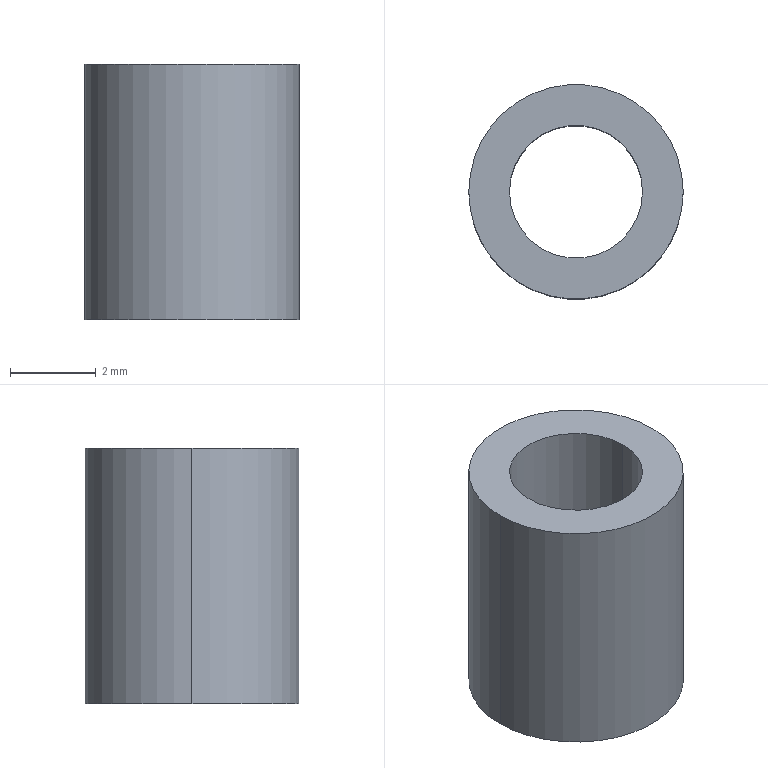Part | SolidWorks | features Extrusion 1 | 1 solid | 6 faces | box 5 x 5 x 5.95 mm | volume 71.919 mm3 | cylinder 4 | plane 2 | commonest cylinder face diameters 3.1 x2 5 x2
STEP:
#1=CARTESIAN_POINT('',(-1.55,0.,5.95));
#2=VERTEX_POINT('',#1);
#3=CARTESIAN_POINT('',(1.55,0.,5.95));
#4=VERTEX_POINT('',#3);
#5=CARTESIAN_POINT('',(0.,0.,5.95));
#6=DIRECTION('',(0.,0.,1.));
#7=DIRECTION('',(1.,0.,0.));
#8=AXIS2_PLACEMENT_3D('',#5,#6,#7);
#9=CIRCLE('',#8,1.55);
#10=EDGE_CURVE('',#2,#4,#9,.T.);
#11=ORIENTED_EDGE('',*,*,#10,.T.);
#12=CARTESIAN_POINT('',(1.55,0.,0.));
#13=VERTEX_POINT('',#12);
#14=CARTESIAN_POINT('',(1.55,0.,5.95));
#15=DIRECTION('',(0.,0.,-1.));
#16=VECTOR('',#15,1000.);
#17=LINE('',#14,#16);
#18=EDGE_CURVE('',#4,#13,#17,.T.);
#19=ORIENTED_EDGE('',*,*,#18,.T.);
#20=CARTESIAN_POINT('',(-1.55,0.,0.));
#21=VERTEX_POINT('',#20);
#22=CARTESIAN_POINT('',(0.,0.,0.));
#23=DIRECTION('',(0.,0.,1.));
#24=DIRECTION('',(1.,0.,0.));
#25=AXIS2_PLACEMENT_3D('',#22,#23,#24);
#26=CIRCLE('',#25,1.55);
#27=EDGE_CURVE('',#21,#13,#26,.T.);
#28=ORIENTED_EDGE('',*,*,#27,.F.);
#29=CARTESIAN_POINT('',(-1.55,0.,5.95));
#30=DIRECTION('',(0.,0.,-1.));
#31=VECTOR('',#30,1000.);
#32=LINE('',#29,#31);
#33=EDGE_CURVE('',#2,#21,#32,.T.);
#34=ORIENTED_EDGE('',*,*,#33,.F.);
#35=EDGE_LOOP('',(#11,#19,#28,#34));
#36=FACE_OUTER_BOUND('',#35,.T.);
#37=CARTESIAN_POINT('',(0.,0.,5.95));
#38=DIRECTION('',(0.,0.,-1.));
#39=DIRECTION('',(-1.,0.,0.));
#40=AXIS2_PLACEMENT_3D('',#37,#38,#39);
#41=CYLINDRICAL_SURFACE('',#40,1.55);
#42=ADVANCED_FACE('',(#36),#41,.F.);
#43=CARTESIAN_POINT('',(2.5,0.,5.95));
#44=VERTEX_POINT('',#43);
#45=CARTESIAN_POINT('',(-2.5,0.,5.95));
#46=VERTEX_POINT('',#45);
#47=CARTESIAN_POINT('',(0.,0.,5.95));
#48=DIRECTION('',(0.,0.,1.));
#49=DIRECTION('',(1.,0.,0.));
#50=AXIS2_PLACEMENT_3D('',#47,#48,#49);
#51=CIRCLE('',#50,2.5);
#52=EDGE_CURVE('',#44,#46,#51,.T.);
#53=ORIENTED_EDGE('',*,*,#52,.F.);
#54=CARTESIAN_POINT('',(2.5,0.,0.));
#55=VERTEX_POINT('',#54);
#56=CARTESIAN_POINT('',(2.5,0.,5.95));
#57=DIRECTION('',(0.,0.,-1.));
#58=VECTOR('',#57,1000.);
#59=LINE('',#56,#58);
#60=EDGE_CURVE('',#44,#55,#59,.T.);
#61=ORIENTED_EDGE('',*,*,#60,.T.);
#62=CARTESIAN_POINT('',(-2.5,0.,0.));
#63=VERTEX_POINT('',#62);
#64=CARTESIAN_POINT('',(0.,0.,0.));
#65=DIRECTION('',(0.,0.,1.));
#66=DIRECTION('',(1.,0.,0.));
#67=AXIS2_PLACEMENT_3D('',#64,#65,#66);
#68=CIRCLE('',#67,2.5);
#69=EDGE_CURVE('',#55,#63,#68,.T.);
#70=ORIENTED_EDGE('',*,*,#69,.T.);
#71=CARTESIAN_POINT('',(-2.5,0.,5.95));
#72=DIRECTION('',(0.,0.,-1.));
#73=VECTOR('',#72,1000.);
#74=LINE('',#71,#73);
#75=EDGE_CURVE('',#46,#63,#74,.T.);
#76=ORIENTED_EDGE('',*,*,#75,.F.);
#77=EDGE_LOOP('',(#53,#61,#70,#76));
#78=FACE_OUTER_BOUND('',#77,.T.);
#79=CARTESIAN_POINT('',(0.,0.,5.95));
#80=DIRECTION('',(0.,0.,-1.));
#81=DIRECTION('',(-1.,0.,0.));
#82=AXIS2_PLACEMENT_3D('',#79,#80,#81);
#83=CYLINDRICAL_SURFACE('',#82,2.5);
#84=ADVANCED_FACE('',(#78),#83,.T.);
#85=CARTESIAN_POINT('',(0.,0.,5.95));
#86=DIRECTION('',(0.,0.,1.));
#87=DIRECTION('',(1.,0.,0.));
#88=AXIS2_PLACEMENT_3D('',#85,#86,#87);
#89=CIRCLE('',#88,2.5);
#90=EDGE_CURVE('',#46,#44,#89,.T.);
#91=ORIENTED_EDGE('',*,*,#90,.T.);
#92=ORIENTED_EDGE('',*,*,#52,.T.);
#93=EDGE_LOOP('',(#91,#92));
#94=FACE_OUTER_BOUND('',#93,.T.);
#95=ORIENTED_EDGE('',*,*,#10,.F.);
#96=CARTESIAN_POINT('',(0.,0.,5.95));
#97=DIRECTION('',(0.,0.,1.));
#98=DIRECTION('',(1.,0.,0.));
#99=AXIS2_PLACEMENT_3D('',#96,#97,#98);
#100=CIRCLE('',#99,1.55);
#101=EDGE_CURVE('',#4,#2,#100,.T.);
#102=ORIENTED_EDGE('',*,*,#101,.F.);
#103=EDGE_LOOP('',(#95,#102));
#104=FACE_BOUND('',#103,.T.);
#105=CARTESIAN_POINT('',(0.,0.,5.95));
#106=DIRECTION('',(0.,0.,1.));
#107=DIRECTION('',(1.,0.,0.));
#108=AXIS2_PLACEMENT_3D('',#105,#106,#107);
#109=PLANE('',#108);
#110=ADVANCED_FACE('',(#94,#104),#109,.T.);
#111=CARTESIAN_POINT('',(0.,0.,0.));
#112=DIRECTION('',(0.,0.,1.));
#113=DIRECTION('',(1.,0.,0.));
#114=AXIS2_PLACEMENT_3D('',#111,#112,#113);
#115=CIRCLE('',#114,2.5);
#116=EDGE_CURVE('',#63,#55,#115,.T.);
#117=ORIENTED_EDGE('',*,*,#116,.F.);
#118=ORIENTED_EDGE('',*,*,#69,.F.);
#119=EDGE_LOOP('',(#117,#118));
#120=FACE_OUTER_BOUND('',#119,.T.);
#121=ORIENTED_EDGE('',*,*,#27,.T.);
#122=CARTESIAN_POINT('',(0.,0.,0.));
#123=DIRECTION('',(0.,0.,1.));
#124=DIRECTION('',(1.,0.,0.));
#125=AXIS2_PLACEMENT_3D('',#122,#123,#124);
#126=CIRCLE('',#125,1.55);
#127=EDGE_CURVE('',#13,#21,#126,.T.);
#128=ORIENTED_EDGE('',*,*,#127,.T.);
#129=EDGE_LOOP('',(#121,#128));
#130=FACE_BOUND('',#129,.T.);
#131=CARTESIAN_POINT('',(0.,0.,0.));
#132=DIRECTION('',(0.,0.,1.));
#133=DIRECTION('',(1.,0.,0.));
#134=AXIS2_PLACEMENT_3D('',#131,#132,#133);
#135=PLANE('',#134);
#136=ADVANCED_FACE('',(#120,#130),#135,.F.);
#137=ORIENTED_EDGE('',*,*,#60,.F.);
#138=ORIENTED_EDGE('',*,*,#90,.F.);
#139=ORIENTED_EDGE('',*,*,#75,.T.);
#140=ORIENTED_EDGE('',*,*,#116,.T.);
#141=EDGE_LOOP('',(#137,#138,#139,#140));
#142=FACE_OUTER_BOUND('',#141,.T.);
#143=CARTESIAN_POINT('',(0.,0.,5.95));
#144=DIRECTION('',(0.,0.,-1.));
#145=DIRECTION('',(-1.,0.,0.));
#146=AXIS2_PLACEMENT_3D('',#143,#144,#145);
#147=CYLINDRICAL_SURFACE('',#146,2.5);
#148=ADVANCED_FACE('',(#142),#147,.T.);
#149=ORIENTED_EDGE('',*,*,#18,.F.);
#150=ORIENTED_EDGE('',*,*,#101,.T.);
#151=ORIENTED_EDGE('',*,*,#33,.T.);
#152=ORIENTED_EDGE('',*,*,#127,.F.);
#153=EDGE_LOOP('',(#149,#150,#151,#152));
#154=FACE_OUTER_BOUND('',#153,.T.);
#155=CARTESIAN_POINT('',(0.,0.,5.95));
#156=DIRECTION('',(0.,0.,-1.));
#157=DIRECTION('',(-1.,0.,0.));
#158=AXIS2_PLACEMENT_3D('',#155,#156,#157);
#159=CYLINDRICAL_SURFACE('',#158,1.55);
#160=ADVANCED_FACE('',(#154),#159,.F.);
#161=CLOSED_SHELL('',(#42,#84,#110,#136,#148,#160));
#162=MANIFOLD_SOLID_BREP('',#161);
#163=CARTESIAN_POINT('',(0.,0.,0.));
#164=DIRECTION('',(0.,0.,1.));
#165=DIRECTION('',(1.,0.,0.));
#166=AXIS2_PLACEMENT_3D('',#163,#164,#165);
#167=(LENGTH_UNIT()NAMED_UNIT(*)SI_UNIT(.MILLI.,.METRE.));
#168=UNCERTAINTY_MEASURE_WITH_UNIT(LENGTH_MEASURE(0.00001),#167,'','');
#169=(NAMED_UNIT(*)PLANE_ANGLE_UNIT()SI_UNIT($,.RADIAN.));
#170=(NAMED_UNIT(*)SI_UNIT($,.STERADIAN.)SOLID_ANGLE_UNIT());
#171=(GEOMETRIC_REPRESENTATION_CONTEXT(3)GLOBAL_UNCERTAINTY_ASSIGNED_CONTEXT((#168))GLOBAL_UNIT_ASSIGNED_CONTEXT((#167,#169,#170))REPRESENTATION_CONTEXT('',''));
#172=ADVANCED_BREP_SHAPE_REPRESENTATION('',(#162,#166),#171);